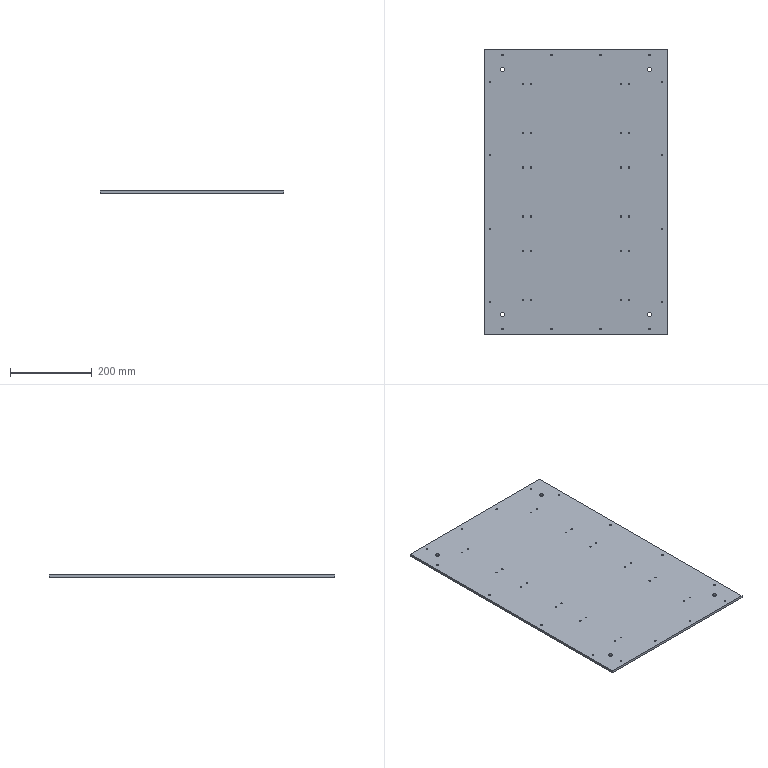Part | SolidWorks | features HoleWzd 2, Cut 1, Extrusion 1 | 1 solid | 94 faces | box 450 x 700 x 6 mm | volume 1886062 mm3 | cylinder 88 | plane 6 | commonest cylinder face diameters 3.3 x80 10 x8